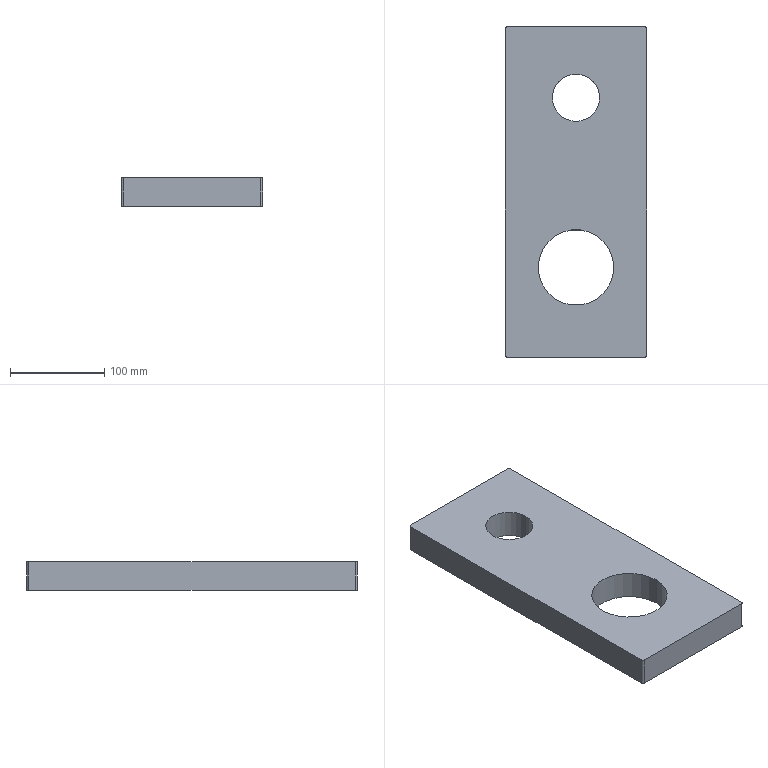Part | SolidWorks | features Extrusion 1, Fillet 1, ICE 1 | 1 solid | 14 faces | box 150 x 350 x 30 mm | volume 1365196 mm3 | cylinder 8 | plane 6 | commonest cylinder face diameters 4 x4 50 x2 80 x2
STEP:
#1=CARTESIAN_POINT('',(-25.,100.,0.));
#2=VERTEX_POINT('',#1);
#3=CARTESIAN_POINT('',(25.,100.,0.));
#4=VERTEX_POINT('',#3);
#5=CARTESIAN_POINT('',(0.,100.,0.));
#6=DIRECTION('',(0.,0.,1.));
#7=DIRECTION('',(1.,0.,0.));
#8=AXIS2_PLACEMENT_3D('',#5,#6,#7);
#9=CIRCLE('',#8,25.);
#10=EDGE_CURVE('',#2,#4,#9,.T.);
#11=ORIENTED_EDGE('',*,*,#10,.F.);
#12=CARTESIAN_POINT('',(-25.,100.,30.));
#13=VERTEX_POINT('',#12);
#14=CARTESIAN_POINT('',(-25.,100.,0.));
#15=DIRECTION('',(0.,0.,1.));
#16=VECTOR('',#15,1000.);
#17=LINE('',#14,#16);
#18=EDGE_CURVE('',#2,#13,#17,.T.);
#19=ORIENTED_EDGE('',*,*,#18,.T.);
#20=CARTESIAN_POINT('',(25.,100.,30.));
#21=VERTEX_POINT('',#20);
#22=CARTESIAN_POINT('',(0.,100.,30.));
#23=DIRECTION('',(0.,0.,1.));
#24=DIRECTION('',(1.,0.,0.));
#25=AXIS2_PLACEMENT_3D('',#22,#23,#24);
#26=CIRCLE('',#25,25.);
#27=EDGE_CURVE('',#13,#21,#26,.T.);
#28=ORIENTED_EDGE('',*,*,#27,.T.);
#29=CARTESIAN_POINT('',(25.,100.,0.));
#30=DIRECTION('',(0.,0.,1.));
#31=VECTOR('',#30,1000.);
#32=LINE('',#29,#31);
#33=EDGE_CURVE('',#4,#21,#32,.T.);
#34=ORIENTED_EDGE('',*,*,#33,.F.);
#35=EDGE_LOOP('',(#11,#19,#28,#34));
#36=FACE_OUTER_BOUND('',#35,.T.);
#37=CARTESIAN_POINT('',(0.,100.,0.));
#38=DIRECTION('',(0.,0.,1.));
#39=DIRECTION('',(1.,0.,0.));
#40=AXIS2_PLACEMENT_3D('',#37,#38,#39);
#41=CYLINDRICAL_SURFACE('',#40,25.);
#42=ADVANCED_FACE('',(#36),#41,.F.);
#43=CARTESIAN_POINT('',(-40.,-80.,0.));
#44=VERTEX_POINT('',#43);
#45=CARTESIAN_POINT('',(40.,-80.,0.));
#46=VERTEX_POINT('',#45);
#47=CARTESIAN_POINT('',(0.,-80.,0.));
#48=DIRECTION('',(0.,0.,1.));
#49=DIRECTION('',(1.,0.,0.));
#50=AXIS2_PLACEMENT_3D('',#47,#48,#49);
#51=CIRCLE('',#50,40.);
#52=EDGE_CURVE('',#44,#46,#51,.T.);
#53=ORIENTED_EDGE('',*,*,#52,.F.);
#54=CARTESIAN_POINT('',(-40.,-80.,30.));
#55=VERTEX_POINT('',#54);
#56=CARTESIAN_POINT('',(-40.,-80.,0.));
#57=DIRECTION('',(0.,0.,1.));
#58=VECTOR('',#57,1000.);
#59=LINE('',#56,#58);
#60=EDGE_CURVE('',#44,#55,#59,.T.);
#61=ORIENTED_EDGE('',*,*,#60,.T.);
#62=CARTESIAN_POINT('',(40.,-80.,30.));
#63=VERTEX_POINT('',#62);
#64=CARTESIAN_POINT('',(0.,-80.,30.));
#65=DIRECTION('',(0.,0.,1.));
#66=DIRECTION('',(1.,0.,0.));
#67=AXIS2_PLACEMENT_3D('',#64,#65,#66);
#68=CIRCLE('',#67,40.);
#69=EDGE_CURVE('',#55,#63,#68,.T.);
#70=ORIENTED_EDGE('',*,*,#69,.T.);
#71=CARTESIAN_POINT('',(40.,-80.,0.));
#72=DIRECTION('',(0.,0.,1.));
#73=VECTOR('',#72,1000.);
#74=LINE('',#71,#73);
#75=EDGE_CURVE('',#46,#63,#74,.T.);
#76=ORIENTED_EDGE('',*,*,#75,.F.);
#77=EDGE_LOOP('',(#53,#61,#70,#76));
#78=FACE_OUTER_BOUND('',#77,.T.);
#79=CARTESIAN_POINT('',(0.,-80.,0.));
#80=DIRECTION('',(0.,0.,1.));
#81=DIRECTION('',(1.,0.,0.));
#82=AXIS2_PLACEMENT_3D('',#79,#80,#81);
#83=CYLINDRICAL_SURFACE('',#82,40.);
#84=ADVANCED_FACE('',(#78),#83,.F.);
#85=CARTESIAN_POINT('',(-75.,173.,0.));
#86=VERTEX_POINT('',#85);
#87=CARTESIAN_POINT('',(-75.,-173.,0.));
#88=VERTEX_POINT('',#87);
#89=CARTESIAN_POINT('',(-75.,175.,0.));
#90=DIRECTION('',(0.,-1.,0.));
#91=VECTOR('',#90,1000.);
#92=LINE('',#89,#91);
#93=EDGE_CURVE('',#86,#88,#92,.T.);
#94=ORIENTED_EDGE('',*,*,#93,.T.);
#95=CARTESIAN_POINT('',(-75.,-173.,30.));
#96=VERTEX_POINT('',#95);
#97=CARTESIAN_POINT('',(-75.,-173.,30.));
#98=DIRECTION('',(0.,0.,1.));
#99=VECTOR('',#98,1000.);
#100=LINE('',#97,#99);
#101=EDGE_CURVE('',#88,#96,#100,.T.);
#102=ORIENTED_EDGE('',*,*,#101,.T.);
#103=CARTESIAN_POINT('',(-75.,173.,30.));
#104=VERTEX_POINT('',#103);
#105=CARTESIAN_POINT('',(-75.,175.,30.));
#106=DIRECTION('',(0.,-1.,0.));
#107=VECTOR('',#106,1000.);
#108=LINE('',#105,#107);
#109=EDGE_CURVE('',#104,#96,#108,.T.);
#110=ORIENTED_EDGE('',*,*,#109,.F.);
#111=CARTESIAN_POINT('',(-75.,173.,30.));
#112=DIRECTION('',(0.,0.,-1.));
#113=VECTOR('',#112,1000.);
#114=LINE('',#111,#113);
#115=EDGE_CURVE('',#104,#86,#114,.T.);
#116=ORIENTED_EDGE('',*,*,#115,.T.);
#117=EDGE_LOOP('',(#94,#102,#110,#116));
#118=FACE_OUTER_BOUND('',#117,.T.);
#119=CARTESIAN_POINT('',(-75.,175.,30.));
#120=DIRECTION('',(1.,0.,0.));
#121=DIRECTION('',(0.,1.,0.));
#122=AXIS2_PLACEMENT_3D('',#119,#120,#121);
#123=PLANE('',#122);
#124=ADVANCED_FACE('',(#118),#123,.F.);
#125=CARTESIAN_POINT('',(-73.,-175.,0.));
#126=VERTEX_POINT('',#125);
#127=CARTESIAN_POINT('',(73.,-175.,0.));
#128=VERTEX_POINT('',#127);
#129=CARTESIAN_POINT('',(75.,-175.,0.));
#130=DIRECTION('',(1.,0.,0.));
#131=VECTOR('',#130,1000.);
#132=LINE('',#129,#131);
#133=EDGE_CURVE('',#126,#128,#132,.T.);
#134=ORIENTED_EDGE('',*,*,#133,.T.);
#135=CARTESIAN_POINT('',(73.,-175.,30.));
#136=VERTEX_POINT('',#135);
#137=CARTESIAN_POINT('',(73.,-175.,30.));
#138=DIRECTION('',(0.,0.,1.));
#139=VECTOR('',#138,1000.);
#140=LINE('',#137,#139);
#141=EDGE_CURVE('',#128,#136,#140,.T.);
#142=ORIENTED_EDGE('',*,*,#141,.T.);
#143=CARTESIAN_POINT('',(-73.,-175.,30.));
#144=VERTEX_POINT('',#143);
#145=CARTESIAN_POINT('',(75.,-175.,30.));
#146=DIRECTION('',(1.,0.,0.));
#147=VECTOR('',#146,1000.);
#148=LINE('',#145,#147);
#149=EDGE_CURVE('',#144,#136,#148,.T.);
#150=ORIENTED_EDGE('',*,*,#149,.F.);
#151=CARTESIAN_POINT('',(-73.,-175.,30.));
#152=DIRECTION('',(0.,0.,-1.));
#153=VECTOR('',#152,1000.);
#154=LINE('',#151,#153);
#155=EDGE_CURVE('',#144,#126,#154,.T.);
#156=ORIENTED_EDGE('',*,*,#155,.T.);
#157=EDGE_LOOP('',(#134,#142,#150,#156));
#158=FACE_OUTER_BOUND('',#157,.T.);
#159=CARTESIAN_POINT('',(75.,-175.,30.));
#160=DIRECTION('',(0.,1.,0.));
#161=DIRECTION('',(-1.,0.,0.));
#162=AXIS2_PLACEMENT_3D('',#159,#160,#161);
#163=PLANE('',#162);
#164=ADVANCED_FACE('',(#158),#163,.F.);
#165=CARTESIAN_POINT('',(75.,-173.,0.));
#166=VERTEX_POINT('',#165);
#167=CARTESIAN_POINT('',(75.,173.,0.));
#168=VERTEX_POINT('',#167);
#169=CARTESIAN_POINT('',(75.,175.,0.));
#170=DIRECTION('',(0.,1.,0.));
#171=VECTOR('',#170,1000.);
#172=LINE('',#169,#171);
#173=EDGE_CURVE('',#166,#168,#172,.T.);
#174=ORIENTED_EDGE('',*,*,#173,.T.);
#175=CARTESIAN_POINT('',(75.,173.,30.));
#176=VERTEX_POINT('',#175);
#177=CARTESIAN_POINT('',(75.,173.,30.));
#178=DIRECTION('',(0.,0.,1.));
#179=VECTOR('',#178,1000.);
#180=LINE('',#177,#179);
#181=EDGE_CURVE('',#168,#176,#180,.T.);
#182=ORIENTED_EDGE('',*,*,#181,.T.);
#183=CARTESIAN_POINT('',(75.,-173.,30.));
#184=VERTEX_POINT('',#183);
#185=CARTESIAN_POINT('',(75.,175.,30.));
#186=DIRECTION('',(0.,1.,0.));
#187=VECTOR('',#186,1000.);
#188=LINE('',#185,#187);
#189=EDGE_CURVE('',#184,#176,#188,.T.);
#190=ORIENTED_EDGE('',*,*,#189,.F.);
#191=CARTESIAN_POINT('',(75.,-173.,30.));
#192=DIRECTION('',(0.,0.,-1.));
#193=VECTOR('',#192,1000.);
#194=LINE('',#191,#193);
#195=EDGE_CURVE('',#184,#166,#194,.T.);
#196=ORIENTED_EDGE('',*,*,#195,.T.);
#197=EDGE_LOOP('',(#174,#182,#190,#196));
#198=FACE_OUTER_BOUND('',#197,.T.);
#199=CARTESIAN_POINT('',(75.,175.,30.));
#200=DIRECTION('',(-1.,0.,0.));
#201=DIRECTION('',(0.,-1.,0.));
#202=AXIS2_PLACEMENT_3D('',#199,#200,#201);
#203=PLANE('',#202);
#204=ADVANCED_FACE('',(#198),#203,.F.);
#205=CARTESIAN_POINT('',(73.,175.,30.));
#206=VERTEX_POINT('',#205);
#207=CARTESIAN_POINT('',(-73.,175.,30.));
#208=VERTEX_POINT('',#207);
#209=CARTESIAN_POINT('',(75.,175.,30.));
#210=DIRECTION('',(-1.,0.,0.));
#211=VECTOR('',#210,1000.);
#212=LINE('',#209,#211);
#213=EDGE_CURVE('',#206,#208,#212,.T.);
#214=ORIENTED_EDGE('',*,*,#213,.F.);
#215=CARTESIAN_POINT('',(73.,175.,0.));
#216=VERTEX_POINT('',#215);
#217=CARTESIAN_POINT('',(73.,175.,30.));
#218=DIRECTION('',(0.,0.,-1.));
#219=VECTOR('',#218,1000.);
#220=LINE('',#217,#219);
#221=EDGE_CURVE('',#206,#216,#220,.T.);
#222=ORIENTED_EDGE('',*,*,#221,.T.);
#223=CARTESIAN_POINT('',(-73.,175.,0.));
#224=VERTEX_POINT('',#223);
#225=CARTESIAN_POINT('',(75.,175.,0.));
#226=DIRECTION('',(-1.,0.,0.));
#227=VECTOR('',#226,1000.);
#228=LINE('',#225,#227);
#229=EDGE_CURVE('',#216,#224,#228,.T.);
#230=ORIENTED_EDGE('',*,*,#229,.T.);
#231=CARTESIAN_POINT('',(-73.,175.,30.));
#232=DIRECTION('',(0.,0.,1.));
#233=VECTOR('',#232,1000.);
#234=LINE('',#231,#233);
#235=EDGE_CURVE('',#224,#208,#234,.T.);
#236=ORIENTED_EDGE('',*,*,#235,.T.);
#237=EDGE_LOOP('',(#214,#222,#230,#236));
#238=FACE_OUTER_BOUND('',#237,.T.);
#239=CARTESIAN_POINT('',(75.,175.,30.));
#240=DIRECTION('',(0.,-1.,0.));
#241=DIRECTION('',(1.,0.,0.));
#242=AXIS2_PLACEMENT_3D('',#239,#240,#241);
#243=PLANE('',#242);
#244=ADVANCED_FACE('',(#238),#243,.F.);
#245=CARTESIAN_POINT('',(0.,100.,30.));
#246=DIRECTION('',(0.,0.,1.));
#247=DIRECTION('',(1.,0.,0.));
#248=AXIS2_PLACEMENT_3D('',#245,#246,#247);
#249=CIRCLE('',#248,25.);
#250=EDGE_CURVE('',#21,#13,#249,.T.);
#251=ORIENTED_EDGE('',*,*,#250,.F.);
#252=ORIENTED_EDGE('',*,*,#27,.F.);
#253=EDGE_LOOP('',(#251,#252));
#254=FACE_BOUND('',#253,.T.);
#255=CARTESIAN_POINT('',(0.,-80.,30.));
#256=DIRECTION('',(0.,0.,1.));
#257=DIRECTION('',(1.,0.,0.));
#258=AXIS2_PLACEMENT_3D('',#255,#256,#257);
#259=CIRCLE('',#258,40.);
#260=EDGE_CURVE('',#63,#55,#259,.T.);
#261=ORIENTED_EDGE('',*,*,#260,.F.);
#262=ORIENTED_EDGE('',*,*,#69,.F.);
#263=EDGE_LOOP('',(#261,#262));
#264=FACE_BOUND('',#263,.T.);
#265=ORIENTED_EDGE('',*,*,#189,.T.);
#266=CARTESIAN_POINT('',(73.,173.,30.));
#267=DIRECTION('',(0.,0.,1.));
#268=DIRECTION('',(-1.,0.,0.));
#269=AXIS2_PLACEMENT_3D('',#266,#267,#268);
#270=CIRCLE('',#269,2.);
#271=EDGE_CURVE('',#176,#206,#270,.T.);
#272=ORIENTED_EDGE('',*,*,#271,.T.);
#273=ORIENTED_EDGE('',*,*,#213,.T.);
#274=CARTESIAN_POINT('',(-73.,173.,30.));
#275=DIRECTION('',(0.,0.,1.));
#276=DIRECTION('',(-1.,0.,0.));
#277=AXIS2_PLACEMENT_3D('',#274,#275,#276);
#278=CIRCLE('',#277,2.);
#279=EDGE_CURVE('',#208,#104,#278,.T.);
#280=ORIENTED_EDGE('',*,*,#279,.T.);
#281=ORIENTED_EDGE('',*,*,#109,.T.);
#282=CARTESIAN_POINT('',(-73.,-173.,30.));
#283=DIRECTION('',(0.,0.,1.));
#284=DIRECTION('',(-1.,0.,0.));
#285=AXIS2_PLACEMENT_3D('',#282,#283,#284);
#286=CIRCLE('',#285,2.);
#287=EDGE_CURVE('',#96,#144,#286,.T.);
#288=ORIENTED_EDGE('',*,*,#287,.T.);
#289=ORIENTED_EDGE('',*,*,#149,.T.);
#290=CARTESIAN_POINT('',(73.,-173.,30.));
#291=DIRECTION('',(0.,0.,1.));
#292=DIRECTION('',(-1.,0.,0.));
#293=AXIS2_PLACEMENT_3D('',#290,#291,#292);
#294=CIRCLE('',#293,2.);
#295=EDGE_CURVE('',#136,#184,#294,.T.);
#296=ORIENTED_EDGE('',*,*,#295,.T.);
#297=EDGE_LOOP('',(#265,#272,#273,#280,#281,#288,#289,#296));
#298=FACE_OUTER_BOUND('',#297,.T.);
#299=CARTESIAN_POINT('',(0.,0.,30.));
#300=DIRECTION('',(0.,0.,-1.));
#301=DIRECTION('',(-1.,0.,0.));
#302=AXIS2_PLACEMENT_3D('',#299,#300,#301);
#303=PLANE('',#302);
#304=ADVANCED_FACE('',(#254,#264,#298),#303,.F.);
#305=CARTESIAN_POINT('',(0.,100.,0.));
#306=DIRECTION('',(0.,0.,1.));
#307=DIRECTION('',(1.,0.,0.));
#308=AXIS2_PLACEMENT_3D('',#305,#306,#307);
#309=CIRCLE('',#308,25.);
#310=EDGE_CURVE('',#4,#2,#309,.T.);
#311=ORIENTED_EDGE('',*,*,#310,.T.);
#312=ORIENTED_EDGE('',*,*,#10,.T.);
#313=EDGE_LOOP('',(#311,#312));
#314=FACE_BOUND('',#313,.T.);
#315=CARTESIAN_POINT('',(0.,-80.,0.));
#316=DIRECTION('',(0.,0.,1.));
#317=DIRECTION('',(1.,0.,0.));
#318=AXIS2_PLACEMENT_3D('',#315,#316,#317);
#319=CIRCLE('',#318,40.);
#320=EDGE_CURVE('',#46,#44,#319,.T.);
#321=ORIENTED_EDGE('',*,*,#320,.T.);
#322=ORIENTED_EDGE('',*,*,#52,.T.);
#323=EDGE_LOOP('',(#321,#322));
#324=FACE_BOUND('',#323,.T.);
#325=ORIENTED_EDGE('',*,*,#229,.F.);
#326=CARTESIAN_POINT('',(73.,173.,0.));
#327=DIRECTION('',(0.,0.,-1.));
#328=DIRECTION('',(-1.,0.,0.));
#329=AXIS2_PLACEMENT_3D('',#326,#327,#328);
#330=CIRCLE('',#329,2.);
#331=EDGE_CURVE('',#216,#168,#330,.T.);
#332=ORIENTED_EDGE('',*,*,#331,.T.);
#333=ORIENTED_EDGE('',*,*,#173,.F.);
#334=CARTESIAN_POINT('',(73.,-173.,0.));
#335=DIRECTION('',(0.,0.,-1.));
#336=DIRECTION('',(-1.,0.,0.));
#337=AXIS2_PLACEMENT_3D('',#334,#335,#336);
#338=CIRCLE('',#337,2.);
#339=EDGE_CURVE('',#166,#128,#338,.T.);
#340=ORIENTED_EDGE('',*,*,#339,.T.);
#341=ORIENTED_EDGE('',*,*,#133,.F.);
#342=CARTESIAN_POINT('',(-73.,-173.,0.));
#343=DIRECTION('',(0.,0.,-1.));
#344=DIRECTION('',(-1.,0.,0.));
#345=AXIS2_PLACEMENT_3D('',#342,#343,#344);
#346=CIRCLE('',#345,2.);
#347=EDGE_CURVE('',#126,#88,#346,.T.);
#348=ORIENTED_EDGE('',*,*,#347,.T.);
#349=ORIENTED_EDGE('',*,*,#93,.F.);
#350=CARTESIAN_POINT('',(-73.,173.,0.));
#351=DIRECTION('',(0.,0.,-1.));
#352=DIRECTION('',(-1.,0.,0.));
#353=AXIS2_PLACEMENT_3D('',#350,#351,#352);
#354=CIRCLE('',#353,2.);
#355=EDGE_CURVE('',#86,#224,#354,.T.);
#356=ORIENTED_EDGE('',*,*,#355,.T.);
#357=EDGE_LOOP('',(#325,#332,#333,#340,#341,#348,#349,#356));
#358=FACE_OUTER_BOUND('',#357,.T.);
#359=CARTESIAN_POINT('',(0.,0.,0.));
#360=DIRECTION('',(0.,0.,-1.));
#361=DIRECTION('',(-1.,0.,0.));
#362=AXIS2_PLACEMENT_3D('',#359,#360,#361);
#363=PLANE('',#362);
#364=ADVANCED_FACE('',(#314,#324,#358),#363,.T.);
#365=ORIENTED_EDGE('',*,*,#60,.F.);
#366=ORIENTED_EDGE('',*,*,#320,.F.);
#367=ORIENTED_EDGE('',*,*,#75,.T.);
#368=ORIENTED_EDGE('',*,*,#260,.T.);
#369=EDGE_LOOP('',(#365,#366,#367,#368));
#370=FACE_OUTER_BOUND('',#369,.T.);
#371=CARTESIAN_POINT('',(0.,-80.,0.));
#372=DIRECTION('',(0.,0.,1.));
#373=DIRECTION('',(1.,0.,0.));
#374=AXIS2_PLACEMENT_3D('',#371,#372,#373);
#375=CYLINDRICAL_SURFACE('',#374,40.);
#376=ADVANCED_FACE('',(#370),#375,.F.);
#377=ORIENTED_EDGE('',*,*,#18,.F.);
#378=ORIENTED_EDGE('',*,*,#310,.F.);
#379=ORIENTED_EDGE('',*,*,#33,.T.);
#380=ORIENTED_EDGE('',*,*,#250,.T.);
#381=EDGE_LOOP('',(#377,#378,#379,#380));
#382=FACE_OUTER_BOUND('',#381,.T.);
#383=CARTESIAN_POINT('',(0.,100.,0.));
#384=DIRECTION('',(0.,0.,1.));
#385=DIRECTION('',(1.,0.,0.));
#386=AXIS2_PLACEMENT_3D('',#383,#384,#385);
#387=CYLINDRICAL_SURFACE('',#386,25.);
#388=ADVANCED_FACE('',(#382),#387,.F.);
#389=ORIENTED_EDGE('',*,*,#271,.F.);
#390=ORIENTED_EDGE('',*,*,#181,.F.);
#391=ORIENTED_EDGE('',*,*,#331,.F.);
#392=ORIENTED_EDGE('',*,*,#221,.F.);
#393=EDGE_LOOP('',(#389,#390,#391,#392));
#394=FACE_OUTER_BOUND('',#393,.T.);
#395=CARTESIAN_POINT('',(73.,173.,30.));
#396=DIRECTION('',(0.,0.,-1.));
#397=DIRECTION('',(-1.,0.,0.));
#398=AXIS2_PLACEMENT_3D('',#395,#396,#397);
#399=CYLINDRICAL_SURFACE('',#398,2.);
#400=ADVANCED_FACE('',(#394),#399,.T.);
#401=ORIENTED_EDGE('',*,*,#295,.F.);
#402=ORIENTED_EDGE('',*,*,#141,.F.);
#403=ORIENTED_EDGE('',*,*,#339,.F.);
#404=ORIENTED_EDGE('',*,*,#195,.F.);
#405=EDGE_LOOP('',(#401,#402,#403,#404));
#406=FACE_OUTER_BOUND('',#405,.T.);
#407=CARTESIAN_POINT('',(73.,-173.,30.));
#408=DIRECTION('',(0.,0.,-1.));
#409=DIRECTION('',(-1.,0.,0.));
#410=AXIS2_PLACEMENT_3D('',#407,#408,#409);
#411=CYLINDRICAL_SURFACE('',#410,2.);
#412=ADVANCED_FACE('',(#406),#411,.T.);
#413=ORIENTED_EDGE('',*,*,#287,.F.);
#414=ORIENTED_EDGE('',*,*,#101,.F.);
#415=ORIENTED_EDGE('',*,*,#347,.F.);
#416=ORIENTED_EDGE('',*,*,#155,.F.);
#417=EDGE_LOOP('',(#413,#414,#415,#416));
#418=FACE_OUTER_BOUND('',#417,.T.);
#419=CARTESIAN_POINT('',(-73.,-173.,30.));
#420=DIRECTION('',(0.,0.,-1.));
#421=DIRECTION('',(-1.,0.,0.));
#422=AXIS2_PLACEMENT_3D('',#419,#420,#421);
#423=CYLINDRICAL_SURFACE('',#422,2.);
#424=ADVANCED_FACE('',(#418),#423,.T.);
#425=ORIENTED_EDGE('',*,*,#279,.F.);
#426=ORIENTED_EDGE('',*,*,#235,.F.);
#427=ORIENTED_EDGE('',*,*,#355,.F.);
#428=ORIENTED_EDGE('',*,*,#115,.F.);
#429=EDGE_LOOP('',(#425,#426,#427,#428));
#430=FACE_OUTER_BOUND('',#429,.T.);
#431=CARTESIAN_POINT('',(-73.,173.,30.));
#432=DIRECTION('',(0.,0.,-1.));
#433=DIRECTION('',(-1.,0.,0.));
#434=AXIS2_PLACEMENT_3D('',#431,#432,#433);
#435=CYLINDRICAL_SURFACE('',#434,2.);
#436=ADVANCED_FACE('',(#430),#435,.T.);
#437=CLOSED_SHELL('',(#42,#84,#124,#164,#204,#244,#304,#364,#376,#388,#400,#412,#424,#436));
#438=MANIFOLD_SOLID_BREP('',#437);
#439=CARTESIAN_POINT('',(0.,0.,0.));
#440=DIRECTION('',(0.,0.,1.));
#441=DIRECTION('',(1.,0.,0.));
#442=AXIS2_PLACEMENT_3D('',#439,#440,#441);
#443=(LENGTH_UNIT()NAMED_UNIT(*)SI_UNIT(.MILLI.,.METRE.));
#444=UNCERTAINTY_MEASURE_WITH_UNIT(LENGTH_MEASURE(0.00001),#443,'','');
#445=(NAMED_UNIT(*)PLANE_ANGLE_UNIT()SI_UNIT($,.RADIAN.));
#446=(NAMED_UNIT(*)SI_UNIT($,.STERADIAN.)SOLID_ANGLE_UNIT());
#447=(GEOMETRIC_REPRESENTATION_CONTEXT(3)GLOBAL_UNCERTAINTY_ASSIGNED_CONTEXT((#444))GLOBAL_UNIT_ASSIGNED_CONTEXT((#443,#445,#446))REPRESENTATION_CONTEXT('',''));
#448=ADVANCED_BREP_SHAPE_REPRESENTATION('',(#438,#442),#447);